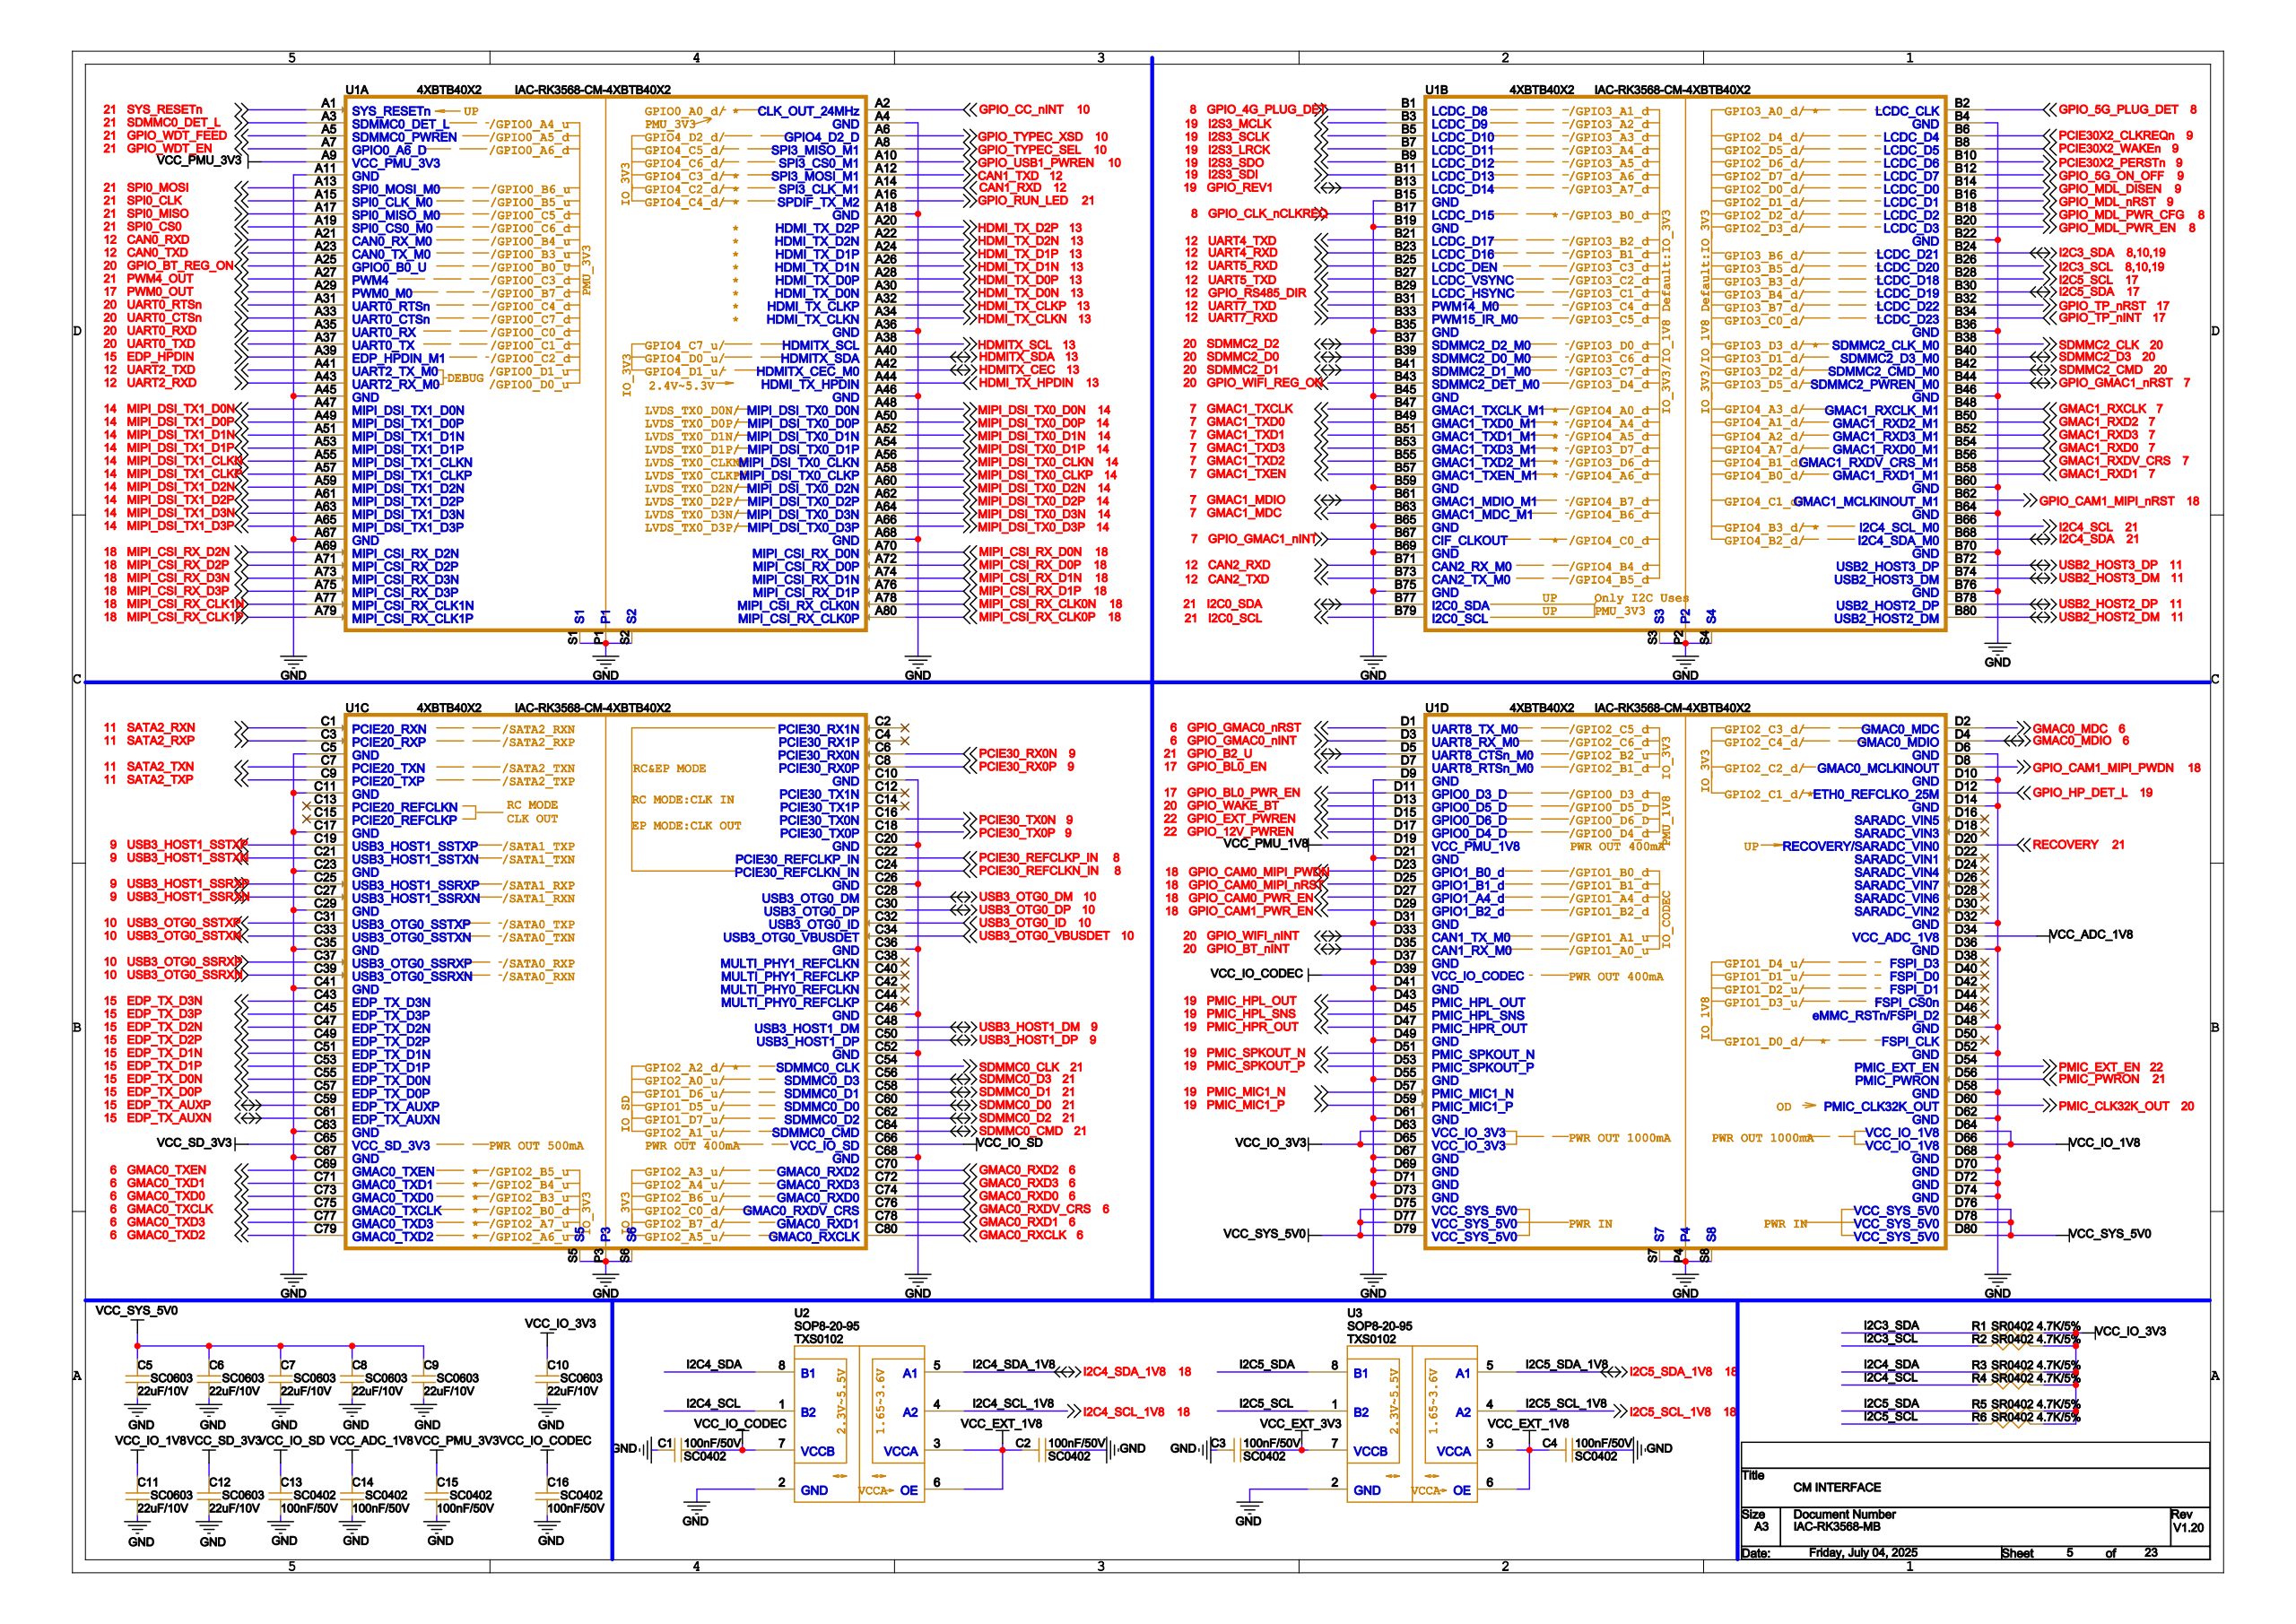Circuit board | Cadence Allegro | 1138 parts | 722 nets | one sheet of the schematic
Parts on this sheet (reference | value | footprint):
C1 | 100nF/50V | SC0402
C2 | 100nF/50V | SC0402
C3 | 100nF/50V | SC0402
C4 | 100nF/50V | SC0402
C5 | 22uF/10V | SC0603
C6 | 22uF/10V | SC0603
C7 | 22uF/10V | SC0603
C8 | 22uF/10V | SC0603
C9 | 22uF/10V | SC0603
C10 | 22uF/10V | SC0603
C11 | 22uF/10V | SC0603
C12 | 22uF/10V | SC0603
C13 | 100nF/50V | SC0402
C14 | 100nF/50V | SC0402
C15 | 100nF/50V | SC0402
C16 | 100nF/50V | SC0402
R1 | 4.7K/5% | SR0402
R2 | 4.7K/5% | SR0402
R3 | 4.7K/5% | SR0402
R4 | 4.7K/5% | SR0402
R5 | 4.7K/5% | SR0402
R6 | 4.7K/5% | SR0402
U1 | 4XBTB40X2 | IAC-RK3568-CM-4XBTB40X2
U2 | TXS0102 | SOP8-20-95
U3 | TXS0102 | SOP8-20-95
Nets of these parts (net: part-pin ...):
GPIO_CAM0_MIPI_PWDN: U1-D23
GPIO_CAM1_MIPI_PWDN: U1-D8
EDP_HPDIN: U1-A39
VCC_EXT_3V3: C3-1 U3-7
GND: C1-2 C2-1 C3-2 C4-1 C5-1 C6-1 C7-1 C8-1 C9-1 C10-1 C11-1 C12-1 C13-1 C14-1 C15-1 C16-1 U2-2 U3-2 U1-A4 U1-A11 U1-A18 U1-A36 U1-A45 U1-A46 U1-A67 U1-A68 U1-B4 U1-B15 U1-B19 U1-B22 U1-B35 U1-B36 U1-B45 U1-B46 U1-B59 U1-B60 U1-B64 U1-B65 U1-B69 U1-B70 U1-B75 U1-B76 U1-C5 U1-C10 U1-C11 U1-C17 U1-C20 U1-C23 U1-C26 U1-C29 U1-C35 U1-C36 U1-C41 U1-C46 U1-C52 U1-C63 U1-C67 U1-C68 U1-D6 U1-D9 U1-D10 U1-D14 U1-D21 U1-D31 U1-D32 U1-D36 U1-D37 U1-D41 U1-D48 U1-D49 U1-D52 U1-D55 U1-D58 U1-D61 U1-D62 U1-D67 U1-D68 U1-D69 U1-D70 U1-D71 U1-D72 U1-D73 U1-D74 U1-P1 U1-P2 U1-P3 U1-P4 U1-S1 U1-S2 U1-S3 U1-S4 U1-S5 U1-S6 U1-S7 U1-S8
PMIC_HPL_OUT: U1-D43
PMIC_HPR_OUT: U1-D47
PMIC_MIC1_P: U1-D59
PMIC_MIC1_N: U1-D57
VCC_SD_3V3: C12-2 U1-C65
RECOVERY: U1-D20
MIPI_DSI_TX0_CLKN: U1-A56
MIPI_DSI_TX0_CLKP: U1-A58
MIPI_DSI_TX1_CLKN: U1-A55
MIPI_DSI_TX1_CLKP: U1-A57
MIPI_CSI_RX_CLK0N: U1-A78
MIPI_CSI_RX_CLK0P: U1-A80
MIPI_CSI_RX_CLK1N: U1-A77
MIPI_CSI_RX_CLK1P: U1-A79
USB3_OTG0_DM: U1-C28
USB3_OTG0_DP: U1-C30
USB2_HOST3_DP: U1-B72
USB2_HOST3_DM: U1-B74
USB2_HOST2_DP: U1-B78
USB2_HOST2_DM: U1-B80
HDMI_TX_D2P: U1-A20
HDMI_TX_D2N: U1-A22
HDMI_TX_D1P: U1-A24
HDMI_TX_D1N: U1-A26
HDMI_TX_D0P: U1-A28
HDMI_TX_D0N: U1-A30
HDMI_TX_CLKP: U1-A32
HDMI_TX_CLKN: U1-A34
EDP_TX_D0N: U1-C55
EDP_TX_D0P: U1-C57
EDP_TX_D1N: U1-C51
EDP_TX_D1P: U1-C53
EDP_TX_D2N: U1-C47
EDP_TX_D2P: U1-C49
EDP_TX_D3N: U1-C43
EDP_TX_D3P: U1-C45
MIPI_CSI_RX_D0N: U1-A70
MIPI_CSI_RX_D0P: U1-A72
MIPI_CSI_RX_D1N: U1-A74
MIPI_CSI_RX_D1P: U1-A76
MIPI_CSI_RX_D2N: U1-A69
MIPI_CSI_RX_D2P: U1-A71
MIPI_CSI_RX_D3N: U1-A73
MIPI_CSI_RX_D3P: U1-A75
MIPI_DSI_TX0_D0N: U1-A48
MIPI_DSI_TX0_D0P: U1-A50
MIPI_DSI_TX0_D1N: U1-A52
MIPI_DSI_TX0_D1P: U1-A54
MIPI_DSI_TX0_D2N: U1-A60
MIPI_DSI_TX0_D2P: U1-A62
MIPI_DSI_TX0_D3N: U1-A64
MIPI_DSI_TX0_D3P: U1-A66
MIPI_DSI_TX1_D0N: U1-A47
MIPI_DSI_TX1_D0P: U1-A49
MIPI_DSI_TX1_D1N: U1-A51
MIPI_DSI_TX1_D1P: U1-A53
MIPI_DSI_TX1_D2N: U1-A59
MIPI_DSI_TX1_D2P: U1-A61
MIPI_DSI_TX1_D3N: U1-A63
MIPI_DSI_TX1_D3P: U1-A65
VCC_EXT_1V8: C2-2 C4-2 U2-3 U2-6 U3-3 U3-6
VCC_IO_1V8: C11-2 U1-D64 U1-D66
HDMITX_SCL: U1-A38
VCC_IO_3V3: C10-2 R1-2 R2-2 R3-2 R4-2 R5-2 R6-2 U1-D63 U1-D65
HDMITX_SDA: U1-A40
HDMITX_CEC: U1-A42
VCC_SYS_5V0: C5-2 C6-2 C7-2 C8-2 C9-2 U1-D75 U1-D76 U1-D77 U1-D78 U1-D79 U1-D80
PCIE30_TX0N: U1-C16
PCIE30_TX0P: U1-C18
PMIC_PWRON: U1-D56
GMAC0_RXCLK: U1-C80
GMAC0_TXCLK: U1-C75
GMAC1_RXCLK: U1-B48
GMAC1_TXCLK: U1-B47
SATA2_TXP: U1-C9
SATA2_TXN: U1-C7
SATA2_RXP: U1-C3
SATA2_RXN: U1-C1
SDMMC2_CLK: U1-B38
SDMMC2_CMD: U1-B42
SDMMC2_D0: U1-B39
SDMMC2_D1: U1-B41
SDMMC2_D2: U1-B37
SDMMC2_D3: U1-B40
GPIO_HP_DET_L: U1-D12
GPIO_RUN_LED: U1-A16
USB3_OTG0_VBUSDET: U1-C34
SPI0_CS0: U1-A19
SPI0_MISO: U1-A17
SPI0_CLK: U1-A15
SPI0_MOSI: U1-A13
I2C4_SDA: R3-1 U2-8 U1-B68
I2C4_SCL: R4-1 U2-1 U1-B66
PWM4_OUT: U1-A27
GPIO_B2_U: U1-D5
PMIC_SPKOUT_P: U1-D53
PMIC_SPKOUT_N: U1-D51
USB3_OTG0_ID: U1-C32
PCIE30_REFCLKP_IN: U1-C22
PCIE30_REFCLKN_IN: U1-C24
USB3_HOST1_DM: U1-C48
USB3_HOST1_DP: U1-C50
CAN0_RXD: U1-A21
CAN1_RXD: U1-A14
CAN2_RXD: U1-B71
VCC_PMU_3V3: C15-2 U1-A9
VCC_IO_CODEC: C1-1 C16-2 U2-7 U1-D39
SDMMC0_DET_L: U1-A3
CAN0_TXD: U1-A23
GPIO_WDT_EN: U1-A7
GPIO_BT_REG_ON: U1-A25
GPIO_TYPEC_XSD: U1-A6
HDMI_TX_HPDIN: U1-A44
PWM0_OUT: U1-A29
GPIO_WDT_FEED: U1-A5
GPIO_USB1_PWREN: U1-A10
GPIO_TYPEC_SEL: U1-A8
CAN1_TXD: U1-A12
UART0_RXD: U1-A35
UART0_TXD: U1-A37
UART2_RXD: U1-A43
UART2_TXD: U1-A41
CAN2_TXD: U1-B73
GMAC1_MDC: U1-B63
GMAC1_MDIO: U1-B61
GMAC1_RXD0: U1-B54
GMAC1_RXD1: U1-B58
GMAC1_RXD2: U1-B50
GMAC1_RXD3: U1-B52
GMAC1_RXDV_CRS: U1-B56
GMAC1_TXD0: U1-B49
GMAC1_TXD1: U1-B51
GMAC1_TXD2: U1-B55
GMAC1_TXD3: U1-B53
GMAC1_TXEN: U1-B57
I2C0_SCL: U1-B79
I2C0_SDA: U1-B77
GPIO_5G_PLUG_DET: U1-B2
GPIO_MDL_DISEN: U1-B14
I2S3_SCLK: U1-B5
I2S3_LRCK: U1-B7
I2S3_SDO: U1-B9
I2S3_SDI: U1-B11
GPIO_REV1: U1-B13
UART4_RXD: U1-B23
UART4_TXD: U1-B21
I2C5_SCL: R6-1 U3-1 U1-B28
I2C5_SDA: R5-1 U3-8 U1-B30
GPIO_MDL_PWR_CFG: U1-B18
I2C3_SCL: R2-1 U1-B26
I2C3_SDA: R1-1 U1-B24
GPIO_MDL_PWR_EN: U1-B20
GPIO_5G_ON_OFF: U1-B12
GPIO_4G_PLUG_DET: U1-B1
I2S3_MCLK: U1-B3
UART5_RXD: U1-B25
GPIO_RS485_DIR: U1-B29
UART5_TXD: U1-B27
UART7_TXD: U1-B31
UART7_RXD: U1-B33
GPIO_WIFI_REG_ON: U1-B43
EDP_TX_AUXN: U1-C61
EDP_TX_AUXP: U1-C59
GMAC0_RXD0: U1-C74
GMAC0_RXD1: U1-C78
GMAC0_RXD2: U1-C70
GMAC0_RXD3: U1-C72
GMAC0_RXDV_CRS: U1-C76
GMAC0_TXD0: U1-C73
GMAC0_TXD1: U1-C71
GMAC0_TXD2: U1-C79
GMAC0_TXD3: U1-C77
GMAC0_TXEN: U1-C69
PCIE30_RX0N: U1-C6
PCIE30_RX0P: U1-C8
SDMMC0_CLK: U1-C54
SDMMC0_CMD: U1-C64
SDMMC0_D0: U1-C60
SDMMC0_D1: U1-C58
SDMMC0_D2: U1-C62
SDMMC0_D3: U1-C56
USB3_HOST1_SSRXN: U1-C27
USB3_HOST1_SSRXP: U1-C25
USB3_HOST1_SSTXN: U1-C21
USB3_HOST1_SSTXP: U1-C19
USB3_OTG0_SSRXN: U1-C39
USB3_OTG0_SSRXP: U1-C37
USB3_OTG0_SSTXN: U1-C33
USB3_OTG0_SSTXP: U1-C31
VCC_IO_SD: C13-2 U1-C66
GMAC0_MDC: U1-D2
GMAC0_MDIO: U1-D4
GPIO_BL0_PWR_EN: U1-D11
GPIO_12V_PWREN: U1-D17
GPIO_WAKE_BT: U1-D13
GPIO_EXT_PWREN: U1-D15
GPIO_CAM0_PWR_EN: U1-D27
GPIO_CAM1_PWR_EN: U1-D29
PMIC_CLK32K_OUT: U1-D60
PMIC_EXT_EN: U1-D54
PMIC_HPL_SNS: U1-D45
GPIO_BL0_EN: U1-D7
VCC_ADC_1V8: C14-2 U1-D34
VCC_PMU_1V8: U1-D19
I2C4_SDA_1V8: U2-5
I2C4_SCL_1V8: U2-4
I2C5_SDA_1V8: U3-5
I2C5_SCL_1V8: U3-4